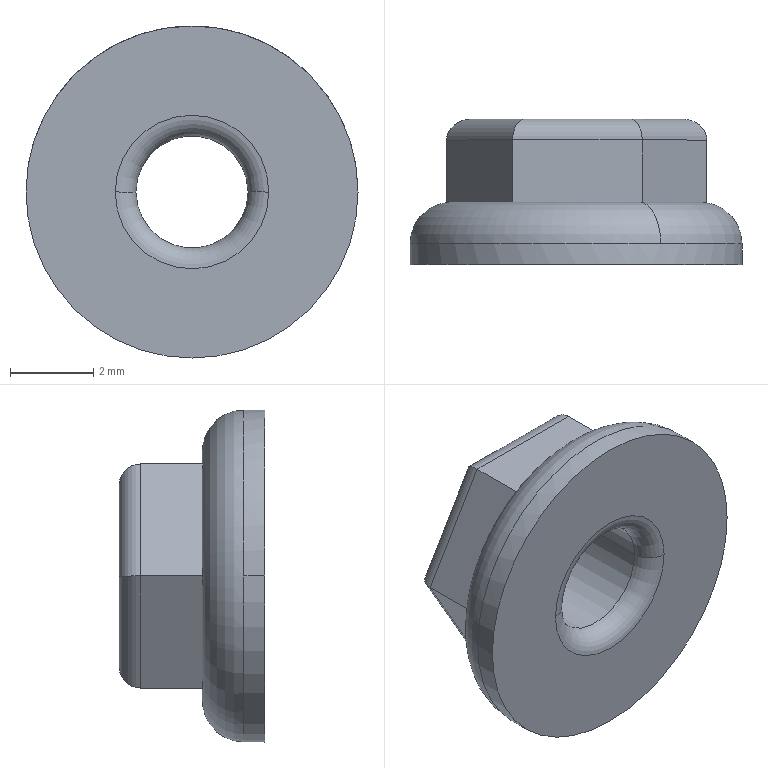Part | STEP file | FANGHUALUOMAO_3_1 | 1 solid | 30 faces | box 8 x 3.5 x 8 mm | volume 99.012 mm3 | plane 14 | cylinder 10 | torus 6 | commonest cylinder face diameters 1 x6 2.7 x2 8 x2
STEP:
#1=CARTESIAN_POINT('',(0.,0.,0.));
#2=DIRECTION('',(0.,0.,1.));
#3=DIRECTION('',(1.,0.,0.));
#4=AXIS2_PLACEMENT_3D('',#1,#2,#3);
#5=CARTESIAN_POINT('',(4.,0.,0.));
#6=VERTEX_POINT('',#5);
#7=CARTESIAN_POINT('',(-4.,0.,0.));
#8=VERTEX_POINT('',#7);
#9=CARTESIAN_POINT('',(0.,0.,0.));
#10=DIRECTION('',(0.,1.,0.));
#11=DIRECTION('',(1.,0.,0.));
#12=AXIS2_PLACEMENT_3D('',#9,#10,#11);
#13=CIRCLE('',#12,4.);
#14=EDGE_CURVE('',#6,#8,#13,.T.);
#15=ORIENTED_EDGE('',*,*,#14,.T.);
#16=CARTESIAN_POINT('',(0.,0.,0.));
#17=DIRECTION('',(0.,1.,0.));
#18=DIRECTION('',(-1.,0.,0.));
#19=AXIS2_PLACEMENT_3D('',#16,#17,#18);
#20=CIRCLE('',#19,4.);
#21=EDGE_CURVE('',#8,#6,#20,.T.);
#22=ORIENTED_EDGE('',*,*,#21,.T.);
#23=EDGE_LOOP('',(#15,#22));
#24=FACE_OUTER_BOUND('',#23,.F.);
#25=CARTESIAN_POINT('',(-1.85,0.,-0.02495));
#26=VERTEX_POINT('',#25);
#27=CARTESIAN_POINT('',(-1.85,0.,0.001234));
#28=VERTEX_POINT('',#27);
#29=CARTESIAN_POINT('',(0.,0.,0.));
#30=DIRECTION('',(0.,1.,0.));
#31=DIRECTION('',(-0.9999,0.,-0.01349));
#32=AXIS2_PLACEMENT_3D('',#29,#30,#31);
#33=CIRCLE('',#32,1.85);
#34=EDGE_CURVE('',#26,#28,#33,.T.);
#35=ORIENTED_EDGE('',*,*,#34,.F.);
#36=CARTESIAN_POINT('',(1.85,0.,-0.001234));
#37=VERTEX_POINT('',#36);
#38=CARTESIAN_POINT('',(0.,0.,0.));
#39=DIRECTION('',(0.,-1.,0.));
#40=DIRECTION('',(-0.9999,0.,-0.01349));
#41=AXIS2_PLACEMENT_3D('',#38,#39,#40);
#42=CIRCLE('',#41,1.85);
#43=EDGE_CURVE('',#26,#37,#42,.T.);
#44=ORIENTED_EDGE('',*,*,#43,.T.);
#45=CARTESIAN_POINT('',(1.85,0.,0.02495));
#46=VERTEX_POINT('',#45);
#47=CARTESIAN_POINT('',(0.,0.,0.));
#48=DIRECTION('',(0.,1.,0.));
#49=DIRECTION('',(0.9999,0.,0.01349));
#50=AXIS2_PLACEMENT_3D('',#47,#48,#49);
#51=CIRCLE('',#50,1.85);
#52=EDGE_CURVE('',#46,#37,#51,.T.);
#53=ORIENTED_EDGE('',*,*,#52,.F.);
#54=CARTESIAN_POINT('',(0.,0.,0.));
#55=DIRECTION('',(0.,-1.,0.));
#56=DIRECTION('',(0.9999,0.,0.01349));
#57=AXIS2_PLACEMENT_3D('',#54,#55,#56);
#58=CIRCLE('',#57,1.85);
#59=EDGE_CURVE('',#46,#28,#58,.T.);
#60=ORIENTED_EDGE('',*,*,#59,.T.);
#61=EDGE_LOOP('',(#35,#44,#53,#60));
#62=FACE_BOUND('',#61,.F.);
#63=CARTESIAN_POINT('',(0.,0.,0.));
#64=DIRECTION('',(0.,1.,0.));
#65=DIRECTION('',(1.,0.,0.));
#66=AXIS2_PLACEMENT_3D('',#63,#64,#65);
#67=PLANE('',#66);
#68=ADVANCED_FACE('',(#24,#62),#67,.F.);
#69=CARTESIAN_POINT('',(-4.,0.5,0.000001668));
#70=VERTEX_POINT('',#69);
#71=CARTESIAN_POINT('',(4.,0.5,0.));
#72=VERTEX_POINT('',#71);
#73=CARTESIAN_POINT('',(0.,0.5,0.));
#74=DIRECTION('',(0.,-1.,0.));
#75=DIRECTION('',(-1.,0.,0.000000417));
#76=AXIS2_PLACEMENT_3D('',#73,#74,#75);
#77=CIRCLE('',#76,4.);
#78=EDGE_CURVE('',#70,#72,#77,.T.);
#79=ORIENTED_EDGE('',*,*,#78,.F.);
#80=CARTESIAN_POINT('',(-4.,0.,0.000001112));
#81=DIRECTION('',(0.,1.,0.000001334));
#82=VECTOR('',#81,0.5);
#83=LINE('',#80,#82);
#84=EDGE_CURVE('',#8,#70,#83,.T.);
#85=ORIENTED_EDGE('',*,*,#84,.F.);
#86=ORIENTED_EDGE('',*,*,#14,.F.);
#87=CARTESIAN_POINT('',(4.,0.,0.));
#88=DIRECTION('',(0.,1.,0.00001117));
#89=VECTOR('',#88,0.5);
#90=LINE('',#87,#89);
#91=EDGE_CURVE('',#6,#72,#90,.T.);
#92=ORIENTED_EDGE('',*,*,#91,.T.);
#93=EDGE_LOOP('',(#79,#85,#86,#92));
#94=FACE_OUTER_BOUND('',#93,.F.);
#95=CARTESIAN_POINT('',(0.,0.,0.));
#96=DIRECTION('',(0.,1.,0.));
#97=DIRECTION('',(1.,0.,0.));
#98=AXIS2_PLACEMENT_3D('',#95,#96,#97);
#99=CYLINDRICAL_SURFACE('',#98,4.);
#100=ADVANCED_FACE('',(#94),#99,.T.);
#101=ORIENTED_EDGE('',*,*,#78,.T.);
#102=CARTESIAN_POINT('',(3.152,1.488,0.000008799));
#103=VERTEX_POINT('',#102);
#104=CARTESIAN_POINT('',(3.,0.5,0.000008374));
#105=DIRECTION('',(0.000002791,0.,-1.));
#106=DIRECTION('',(0.1523,0.9883,0.000000425));
#107=AXIS2_PLACEMENT_3D('',#104,#105,#106);
#108=CIRCLE('',#107,1.);
#109=EDGE_CURVE('',#103,#72,#108,.T.);
#110=ORIENTED_EDGE('',*,*,#109,.F.);
#111=CARTESIAN_POINT('',(2.987,1.5,-0.2804));
#112=VERTEX_POINT('',#111);
#113=CARTESIAN_POINT('',(3.005,1.5,-0.2493));
#114=CARTESIAN_POINT('',(3.042,1.499,-0.1872));
#115=CARTESIAN_POINT('',(3.097,1.496,-0.09395));
#116=CARTESIAN_POINT('',(3.134,1.491,-0.03136));
#117=CARTESIAN_POINT('',(3.152,1.488,0.000005525));
#118=B_SPLINE_CURVE_WITH_KNOTS('',3,(#111,#113,#114,#115,#116,#117),.UNSPECIFIED.,.F.,.F.,(4,1,1,4),(0.,0.3333,0.6667,1.),.UNSPECIFIED.);
#119=EDGE_CURVE('',#112,#103,#118,.T.);
#120=ORIENTED_EDGE('',*,*,#119,.F.);
#121=CARTESIAN_POINT('',(1.689,1.5,-2.479));
#122=VERTEX_POINT('',#121);
#123=CARTESIAN_POINT('',(0.,1.5,0.));
#124=DIRECTION('',(0.,-1.,0.));
#125=DIRECTION('',(0.563,0.,-0.8264));
#126=AXIS2_PLACEMENT_3D('',#123,#124,#125);
#127=CIRCLE('',#126,3.);
#128=EDGE_CURVE('',#122,#112,#127,.T.);
#129=ORIENTED_EDGE('',*,*,#128,.F.);
#130=CARTESIAN_POINT('',(1.559,1.493,-2.7));
#131=VERTEX_POINT('',#130);
#132=CARTESIAN_POINT('',(1.689,1.5,-2.479));
#133=CARTESIAN_POINT('',(1.674,1.5,-2.504));
#134=CARTESIAN_POINT('',(1.645,1.5,-2.554));
#135=CARTESIAN_POINT('',(1.602,1.497,-2.628));
#136=CARTESIAN_POINT('',(1.573,1.495,-2.676));
#137=B_SPLINE_CURVE_WITH_KNOTS('',3,(#132,#133,#134,#135,#136,#130),.UNSPECIFIED.,.F.,.F.,(4,1,1,4),(0.,0.3333,0.6667,1.),.UNSPECIFIED.);
#138=EDGE_CURVE('',#122,#131,#137,.T.);
#139=ORIENTED_EDGE('',*,*,#138,.T.);
#140=CARTESIAN_POINT('',(1.308,1.5,-2.7));
#141=VERTEX_POINT('',#140);
#142=CARTESIAN_POINT('',(1.335,1.5,-2.7));
#143=CARTESIAN_POINT('',(1.391,1.5,-2.7));
#144=CARTESIAN_POINT('',(1.475,1.497,-2.7));
#145=CARTESIAN_POINT('',(1.531,1.495,-2.7));
#146=CARTESIAN_POINT('',(1.559,1.493,-2.7));
#147=B_SPLINE_CURVE_WITH_KNOTS('',3,(#140,#142,#143,#144,#145,#146),.UNSPECIFIED.,.F.,.F.,(4,1,1,4),(0.,0.3333,0.6667,1.),.UNSPECIFIED.);
#148=EDGE_CURVE('',#141,#131,#147,.T.);
#149=ORIENTED_EDGE('',*,*,#148,.F.);
#150=CARTESIAN_POINT('',(-0.004458,1.5,-3.));
#151=VERTEX_POINT('',#150);
#152=CARTESIAN_POINT('',(0.,1.5,0.));
#153=DIRECTION('',(0.,-1.,0.));
#154=DIRECTION('',(-0.001486,0.,-1.));
#155=AXIS2_PLACEMENT_3D('',#152,#153,#154);
#156=CIRCLE('',#155,3.);
#157=EDGE_CURVE('',#151,#141,#156,.T.);
#158=ORIENTED_EDGE('',*,*,#157,.F.);
#159=CARTESIAN_POINT('',(-1.308,1.5,-2.7));
#160=VERTEX_POINT('',#159);
#161=CARTESIAN_POINT('',(0.,1.5,0.));
#162=DIRECTION('',(0.,-1.,0.));
#163=DIRECTION('',(-0.4359,0.,-0.9));
#164=AXIS2_PLACEMENT_3D('',#161,#162,#163);
#165=CIRCLE('',#164,3.);
#166=EDGE_CURVE('',#160,#151,#165,.T.);
#167=ORIENTED_EDGE('',*,*,#166,.F.);
#168=CARTESIAN_POINT('',(-1.559,1.493,-2.7));
#169=VERTEX_POINT('',#168);
#170=CARTESIAN_POINT('',(-1.531,1.495,-2.7));
#171=CARTESIAN_POINT('',(-1.475,1.497,-2.7));
#172=CARTESIAN_POINT('',(-1.391,1.5,-2.7));
#173=CARTESIAN_POINT('',(-1.335,1.5,-2.7));
#174=CARTESIAN_POINT('',(-1.308,1.5,-2.7));
#175=B_SPLINE_CURVE_WITH_KNOTS('',3,(#168,#170,#171,#172,#173,#174),.UNSPECIFIED.,.F.,.F.,(4,1,1,4),(0.,0.3333,0.6667,1.),.UNSPECIFIED.);
#176=EDGE_CURVE('',#169,#160,#175,.T.);
#177=ORIENTED_EDGE('',*,*,#176,.F.);
#178=CARTESIAN_POINT('',(-1.684,1.5,-2.482));
#179=VERTEX_POINT('',#178);
#180=CARTESIAN_POINT('',(-1.671,1.5,-2.507));
#181=CARTESIAN_POINT('',(-1.643,1.5,-2.555));
#182=CARTESIAN_POINT('',(-1.601,1.497,-2.627));
#183=CARTESIAN_POINT('',(-1.573,1.495,-2.676));
#184=CARTESIAN_POINT('',(-1.559,1.493,-2.7));
#185=B_SPLINE_CURVE_WITH_KNOTS('',3,(#178,#180,#181,#182,#183,#184),.UNSPECIFIED.,.F.,.F.,(4,1,1,4),(0.,0.3333,0.6667,1.),.UNSPECIFIED.);
#186=EDGE_CURVE('',#179,#169,#185,.T.);
#187=ORIENTED_EDGE('',*,*,#186,.F.);
#188=CARTESIAN_POINT('',(-2.992,1.5,-0.2175));
#189=VERTEX_POINT('',#188);
#190=CARTESIAN_POINT('',(0.,1.5,0.));
#191=DIRECTION('',(0.,-1.,0.));
#192=DIRECTION('',(-0.9974,0.,-0.07251));
#193=AXIS2_PLACEMENT_3D('',#190,#191,#192);
#194=CIRCLE('',#193,3.);
#195=EDGE_CURVE('',#189,#179,#194,.T.);
#196=ORIENTED_EDGE('',*,*,#195,.F.);
#197=CARTESIAN_POINT('',(-3.118,1.493,0.0002294));
#198=VERTEX_POINT('',#197);
#199=CARTESIAN_POINT('',(-3.104,1.495,-0.0243));
#200=CARTESIAN_POINT('',(-3.075,1.497,-0.07314));
#201=CARTESIAN_POINT('',(-3.034,1.5,-0.1456));
#202=CARTESIAN_POINT('',(-3.006,1.5,-0.1936));
#203=CARTESIAN_POINT('',(-2.992,1.5,-0.2175));
#204=B_SPLINE_CURVE_WITH_KNOTS('',3,(#197,#199,#200,#201,#202,#203),.UNSPECIFIED.,.F.,.F.,(4,1,1,4),(0.,0.3333,0.6667,1.),.UNSPECIFIED.);
#205=EDGE_CURVE('',#198,#189,#204,.T.);
#206=ORIENTED_EDGE('',*,*,#205,.F.);
#207=CARTESIAN_POINT('',(-2.992,1.5,0.2127));
#208=VERTEX_POINT('',#207);
#209=CARTESIAN_POINT('',(-3.006,1.5,0.1891));
#210=CARTESIAN_POINT('',(-3.034,1.5,0.1418));
#211=CARTESIAN_POINT('',(-3.076,1.497,0.07108));
#212=CARTESIAN_POINT('',(-3.104,1.495,0.02384));
#213=CARTESIAN_POINT('',(-3.118,1.493,0.0002294));
#214=B_SPLINE_CURVE_WITH_KNOTS('',3,(#207,#209,#210,#211,#212,#213),.UNSPECIFIED.,.F.,.F.,(4,1,1,4),(0.,0.3333,0.6667,1.),.UNSPECIFIED.);
#215=EDGE_CURVE('',#208,#198,#214,.T.);
#216=ORIENTED_EDGE('',*,*,#215,.F.);
#217=CARTESIAN_POINT('',(-1.633,1.5,2.517));
#218=VERTEX_POINT('',#217);
#219=CARTESIAN_POINT('',(0.,1.5,0.));
#220=DIRECTION('',(0.,-1.,0.));
#221=DIRECTION('',(-0.5442,0.,0.839));
#222=AXIS2_PLACEMENT_3D('',#219,#220,#221);
#223=CIRCLE('',#222,3.);
#224=EDGE_CURVE('',#218,#208,#223,.T.);
#225=ORIENTED_EDGE('',*,*,#224,.F.);
#226=CARTESIAN_POINT('',(-1.524,1.495,2.7));
#227=VERTEX_POINT('',#226);
#228=CARTESIAN_POINT('',(-1.537,1.496,2.679));
#229=CARTESIAN_POINT('',(-1.561,1.498,2.638));
#230=CARTESIAN_POINT('',(-1.597,1.5,2.577));
#231=CARTESIAN_POINT('',(-1.621,1.5,2.537));
#232=CARTESIAN_POINT('',(-1.633,1.5,2.517));
#233=B_SPLINE_CURVE_WITH_KNOTS('',3,(#226,#228,#229,#230,#231,#232),.UNSPECIFIED.,.F.,.F.,(4,1,1,4),(0.,0.3333,0.6667,1.),.UNSPECIFIED.);
#234=EDGE_CURVE('',#227,#218,#233,.T.);
#235=ORIENTED_EDGE('',*,*,#234,.F.);
#236=CARTESIAN_POINT('',(-1.308,1.5,2.7));
#237=VERTEX_POINT('',#236);
#238=CARTESIAN_POINT('',(-1.524,1.495,2.7));
#239=CARTESIAN_POINT('',(-1.501,1.496,2.7));
#240=CARTESIAN_POINT('',(-1.453,1.498,2.7));
#241=CARTESIAN_POINT('',(-1.381,1.5,2.7));
#242=CARTESIAN_POINT('',(-1.332,1.5,2.7));
#243=B_SPLINE_CURVE_WITH_KNOTS('',3,(#238,#239,#240,#241,#242,#236),.UNSPECIFIED.,.F.,.F.,(4,1,1,4),(0.,0.3333,0.6667,1.),.UNSPECIFIED.);
#244=EDGE_CURVE('',#227,#237,#243,.T.);
#245=ORIENTED_EDGE('',*,*,#244,.T.);
#246=CARTESIAN_POINT('',(0.004458,1.5,3.));
#247=VERTEX_POINT('',#246);
#248=CARTESIAN_POINT('',(0.,1.5,0.));
#249=DIRECTION('',(0.,-1.,0.));
#250=DIRECTION('',(0.001486,0.,1.));
#251=AXIS2_PLACEMENT_3D('',#248,#249,#250);
#252=CIRCLE('',#251,3.);
#253=EDGE_CURVE('',#247,#237,#252,.T.);
#254=ORIENTED_EDGE('',*,*,#253,.F.);
#255=CARTESIAN_POINT('',(1.308,1.5,2.7));
#256=VERTEX_POINT('',#255);
#257=CARTESIAN_POINT('',(0.,1.5,0.));
#258=DIRECTION('',(0.,-1.,0.));
#259=DIRECTION('',(0.4359,0.,0.9));
#260=AXIS2_PLACEMENT_3D('',#257,#258,#259);
#261=CIRCLE('',#260,3.);
#262=EDGE_CURVE('',#256,#247,#261,.T.);
#263=ORIENTED_EDGE('',*,*,#262,.F.);
#264=CARTESIAN_POINT('',(1.593,1.491,2.7));
#265=VERTEX_POINT('',#264);
#266=CARTESIAN_POINT('',(1.561,1.493,2.7));
#267=CARTESIAN_POINT('',(1.498,1.497,2.7));
#268=CARTESIAN_POINT('',(1.402,1.499,2.7));
#269=CARTESIAN_POINT('',(1.339,1.5,2.7));
#270=CARTESIAN_POINT('',(1.308,1.5,2.7));
#271=B_SPLINE_CURVE_WITH_KNOTS('',3,(#264,#266,#267,#268,#269,#270),.UNSPECIFIED.,.F.,.F.,(4,1,1,4),(0.,0.3333,0.6667,1.),.UNSPECIFIED.);
#272=EDGE_CURVE('',#265,#256,#271,.T.);
#273=ORIENTED_EDGE('',*,*,#272,.F.);
#274=CARTESIAN_POINT('',(1.597,1.491,2.693));
#275=VERTEX_POINT('',#274);
#276=CARTESIAN_POINT('',(1.597,1.491,2.694));
#277=CARTESIAN_POINT('',(1.596,1.491,2.695));
#278=CARTESIAN_POINT('',(1.595,1.491,2.698));
#279=CARTESIAN_POINT('',(1.594,1.491,2.699));
#280=CARTESIAN_POINT('',(1.593,1.491,2.7));
#281=B_SPLINE_CURVE_WITH_KNOTS('',3,(#274,#276,#277,#278,#279,#280),.UNSPECIFIED.,.F.,.F.,(4,1,1,4),(0.,0.3333,0.6667,1.),.UNSPECIFIED.);
#282=EDGE_CURVE('',#275,#265,#281,.T.);
#283=ORIENTED_EDGE('',*,*,#282,.F.);
#284=CARTESIAN_POINT('',(2.041,0.5,3.44));
#285=VERTEX_POINT('',#284);
#286=CARTESIAN_POINT('',(1.53,0.5,2.58));
#287=DIRECTION('',(0.8601,0.,-0.5101));
#288=DIRECTION('',(0.06699,0.9913,0.1129));
#289=AXIS2_PLACEMENT_3D('',#286,#287,#288);
#290=CIRCLE('',#289,1.);
#291=EDGE_CURVE('',#275,#285,#290,.T.);
#292=ORIENTED_EDGE('',*,*,#291,.T.);
#293=CARTESIAN_POINT('',(0.,0.5,0.));
#294=DIRECTION('',(0.,-1.,0.));
#295=DIRECTION('',(0.5101,0.,0.8601));
#296=AXIS2_PLACEMENT_3D('',#293,#294,#295);
#297=CIRCLE('',#296,4.);
#298=EDGE_CURVE('',#285,#70,#297,.T.);
#299=ORIENTED_EDGE('',*,*,#298,.T.);
#300=EDGE_LOOP('',(#101,#110,#120,#129,#139,#149,#158,#167,#177,#187,#196,#206,#216,#225,#235,#245,#254,#263,#273,#283,#292,#299));
#301=FACE_OUTER_BOUND('',#300,.F.);
#302=CARTESIAN_POINT('',(0.,0.5,0.));
#303=DIRECTION('',(0.,1.,0.));
#304=DIRECTION('',(-0.001486,0.,-1.));
#305=AXIS2_PLACEMENT_3D('',#302,#303,#304);
#306=TOROIDAL_SURFACE('',#305,3.,1.);
#307=ADVANCED_FACE('',(#301),#306,.T.);
#308=CARTESIAN_POINT('',(0.,0.5,0.));
#309=DIRECTION('',(0.,-1.,0.));
#310=DIRECTION('',(1.,0.,0.));
#311=AXIS2_PLACEMENT_3D('',#308,#309,#310);
#312=CIRCLE('',#311,4.);
#313=EDGE_CURVE('',#72,#285,#312,.T.);
#314=ORIENTED_EDGE('',*,*,#313,.T.);
#315=ORIENTED_EDGE('',*,*,#291,.F.);
#316=CARTESIAN_POINT('',(1.742,1.5,2.442));
#317=VERTEX_POINT('',#316);
#318=CARTESIAN_POINT('',(1.726,1.5,2.47));
#319=CARTESIAN_POINT('',(1.694,1.499,2.526));
#320=CARTESIAN_POINT('',(1.646,1.497,2.609));
#321=CARTESIAN_POINT('',(1.614,1.493,2.665));
#322=CARTESIAN_POINT('',(1.597,1.491,2.693));
#323=B_SPLINE_CURVE_WITH_KNOTS('',3,(#316,#318,#319,#320,#321,#322),.UNSPECIFIED.,.F.,.F.,(4,1,1,4),(0.,0.3333,0.6667,1.),.UNSPECIFIED.);
#324=EDGE_CURVE('',#317,#275,#323,.T.);
#325=ORIENTED_EDGE('',*,*,#324,.F.);
#326=CARTESIAN_POINT('',(2.986,1.5,0.2878));
#327=VERTEX_POINT('',#326);
#328=CARTESIAN_POINT('',(0.,1.5,0.));
#329=DIRECTION('',(0.,-1.,0.));
#330=DIRECTION('',(0.9954,0.,0.09594));
#331=AXIS2_PLACEMENT_3D('',#328,#329,#330);
#332=CIRCLE('',#331,3.);
#333=EDGE_CURVE('',#327,#317,#332,.T.);
#334=ORIENTED_EDGE('',*,*,#333,.F.);
#335=CARTESIAN_POINT('',(3.152,1.488,0.000005525));
#336=CARTESIAN_POINT('',(3.134,1.491,0.03193));
#337=CARTESIAN_POINT('',(3.097,1.496,0.09583));
#338=CARTESIAN_POINT('',(3.042,1.499,0.1917));
#339=CARTESIAN_POINT('',(3.005,1.5,0.2558));
#340=CARTESIAN_POINT('',(2.986,1.5,0.2878));
#341=B_SPLINE_CURVE_WITH_KNOTS('',3,(#335,#336,#337,#338,#339,#340),.UNSPECIFIED.,.F.,.F.,(4,1,1,4),(0.,0.3333,0.6667,1.),.UNSPECIFIED.);
#342=EDGE_CURVE('',#103,#327,#341,.T.);
#343=ORIENTED_EDGE('',*,*,#342,.F.);
#344=ORIENTED_EDGE('',*,*,#109,.T.);
#345=EDGE_LOOP('',(#314,#315,#325,#334,#343,#344));
#346=FACE_OUTER_BOUND('',#345,.F.);
#347=CARTESIAN_POINT('',(0.,0.5,0.));
#348=DIRECTION('',(0.,1.,0.));
#349=DIRECTION('',(-0.001486,0.,-1.));
#350=AXIS2_PLACEMENT_3D('',#347,#348,#349);
#351=TOROIDAL_SURFACE('',#350,3.,1.);
#352=ADVANCED_FACE('',(#346),#351,.T.);
#353=ORIENTED_EDGE('',*,*,#313,.F.);
#354=ORIENTED_EDGE('',*,*,#91,.F.);
#355=ORIENTED_EDGE('',*,*,#21,.F.);
#356=ORIENTED_EDGE('',*,*,#84,.T.);
#357=ORIENTED_EDGE('',*,*,#298,.F.);
#358=EDGE_LOOP('',(#353,#354,#355,#356,#357));
#359=FACE_OUTER_BOUND('',#358,.F.);
#360=CARTESIAN_POINT('',(0.,0.,0.));
#361=DIRECTION('',(0.,1.,0.));
#362=DIRECTION('',(1.,0.,0.));
#363=AXIS2_PLACEMENT_3D('',#360,#361,#362);
#364=CYLINDRICAL_SURFACE('',#363,4.);
#365=ADVANCED_FACE('',(#359),#364,.T.);
#366=CARTESIAN_POINT('',(3.152,3.,0.000001431));
#367=VERTEX_POINT('',#366);
#368=CARTESIAN_POINT('',(3.152,1.488,0.000005525));
#369=DIRECTION('',(0.000000206,1.,-0.000002708));
#370=VECTOR('',#369,1.512);
#371=LINE('',#368,#370);
#372=EDGE_CURVE('',#103,#367,#371,.T.);
#373=ORIENTED_EDGE('',*,*,#372,.F.);
#374=ORIENTED_EDGE('',*,*,#342,.T.);
#375=CARTESIAN_POINT('',(1.742,1.5,2.442));
#376=DIRECTION('',(0.5,0.,-0.866));
#377=VECTOR('',#376,2.488);
#378=LINE('',#375,#377);
#379=EDGE_CURVE('',#317,#327,#378,.T.);
#380=ORIENTED_EDGE('',*,*,#379,.F.);
#381=ORIENTED_EDGE('',*,*,#324,.T.);
#382=ORIENTED_EDGE('',*,*,#282,.T.);
#383=CARTESIAN_POINT('',(1.593,3.,2.7));
#384=VERTEX_POINT('',#383);
#385=CARTESIAN_POINT('',(1.593,1.491,2.7));
#386=DIRECTION('',(0.000001295,1.,0.000002194));
#387=VECTOR('',#386,1.509);
#388=LINE('',#385,#387);
#389=EDGE_CURVE('',#265,#384,#388,.T.);
#390=ORIENTED_EDGE('',*,*,#389,.T.);
#391=CARTESIAN_POINT('',(3.152,3.,0.000001431));
#392=DIRECTION('',(-0.5,0.,0.866));
#393=VECTOR('',#392,3.118);
#394=LINE('',#391,#393);
#395=EDGE_CURVE('',#367,#384,#394,.T.);
#396=ORIENTED_EDGE('',*,*,#395,.F.);
#397=EDGE_LOOP('',(#373,#374,#380,#381,#382,#390,#396));
#398=FACE_OUTER_BOUND('',#397,.F.);
#399=CARTESIAN_POINT('',(1.593,1.5,2.7));
#400=DIRECTION('',(0.866,0.,0.5));
#401=DIRECTION('',(0.5,0.,-0.866));
#402=AXIS2_PLACEMENT_3D('',#399,#400,#401);
#403=PLANE('',#402);
#404=ADVANCED_FACE('',(#398),#403,.T.);
#405=CARTESIAN_POINT('',(1.559,3.,-2.7));
#406=VERTEX_POINT('',#405);
#407=CARTESIAN_POINT('',(1.559,1.493,-2.7));
#408=DIRECTION('',(0.,1.,0.));
#409=VECTOR('',#408,1.507);
#410=LINE('',#407,#409);
#411=EDGE_CURVE('',#131,#406,#410,.T.);
#412=ORIENTED_EDGE('',*,*,#411,.F.);
#413=ORIENTED_EDGE('',*,*,#138,.F.);
#414=CARTESIAN_POINT('',(2.987,1.5,-0.2804));
#415=DIRECTION('',(-0.5083,0.,-0.8612));
#416=VECTOR('',#415,2.553);
#417=LINE('',#414,#416);
#418=EDGE_CURVE('',#112,#122,#417,.T.);
#419=ORIENTED_EDGE('',*,*,#418,.F.);
#420=ORIENTED_EDGE('',*,*,#119,.T.);
#421=ORIENTED_EDGE('',*,*,#372,.T.);
#422=CARTESIAN_POINT('',(1.559,3.,-2.7));
#423=DIRECTION('',(0.5083,0.,0.8612));
#424=VECTOR('',#423,3.135);
#425=LINE('',#422,#424);
#426=EDGE_CURVE('',#406,#367,#425,.T.);
#427=ORIENTED_EDGE('',*,*,#426,.F.);
#428=EDGE_LOOP('',(#412,#413,#419,#420,#421,#427));
#429=FACE_OUTER_BOUND('',#428,.F.);
#430=CARTESIAN_POINT('',(3.152,1.5,0.));
#431=DIRECTION('',(0.8612,0.,-0.5083));
#432=DIRECTION('',(-0.5083,0.,-0.8612));
#433=AXIS2_PLACEMENT_3D('',#430,#431,#432);
#434=PLANE('',#433);
#435=ADVANCED_FACE('',(#429),#434,.T.);
#436=CARTESIAN_POINT('',(-1.559,3.,-2.7));
#437=VERTEX_POINT('',#436);
#438=CARTESIAN_POINT('',(-1.559,1.493,-2.7));
#439=DIRECTION('',(-0.000000306,1.,0.000000029));
#440=VECTOR('',#439,1.507);
#441=LINE('',#438,#440);
#442=EDGE_CURVE('',#169,#437,#441,.T.);
#443=ORIENTED_EDGE('',*,*,#442,.F.);
#444=ORIENTED_EDGE('',*,*,#176,.T.);
#445=CARTESIAN_POINT('',(1.308,1.5,-2.7));
#446=DIRECTION('',(-1.,0.,0.000000015));
#447=VECTOR('',#446,2.615);
#448=LINE('',#445,#447);
#449=EDGE_CURVE('',#141,#160,#448,.T.);
#450=ORIENTED_EDGE('',*,*,#449,.F.);
#451=ORIENTED_EDGE('',*,*,#148,.T.);
#452=ORIENTED_EDGE('',*,*,#411,.T.);
#453=CARTESIAN_POINT('',(-1.559,3.,-2.7));
#454=DIRECTION('',(1.,0.,0.00000007));
#455=VECTOR('',#454,3.118);
#456=LINE('',#453,#455);
#457=EDGE_CURVE('',#437,#406,#456,.T.);
#458=ORIENTED_EDGE('',*,*,#457,.F.);
#459=EDGE_LOOP('',(#443,#444,#450,#451,#452,#458));
#460=FACE_OUTER_BOUND('',#459,.F.);
#461=CARTESIAN_POINT('',(1.559,1.5,-2.7));
#462=DIRECTION('',(0.,0.,-1.));
#463=DIRECTION('',(-1.,0.,0.));
#464=AXIS2_PLACEMENT_3D('',#461,#462,#463);
#465=PLANE('',#464);
#466=ADVANCED_FACE('',(#460),#465,.T.);
#467=CARTESIAN_POINT('',(-3.118,3.,0.0002368));
#468=VERTEX_POINT('',#467);
#469=CARTESIAN_POINT('',(-3.118,3.,0.0002368));
#470=DIRECTION('',(0.000002242,-1.,-0.000004906));
#471=VECTOR('',#470,1.507);
#472=LINE('',#469,#471);
#473=EDGE_CURVE('',#468,#198,#472,.T.);
#474=ORIENTED_EDGE('',*,*,#473,.T.);
#475=ORIENTED_EDGE('',*,*,#205,.T.);
#476=CARTESIAN_POINT('',(-1.684,1.5,-2.482));
#477=DIRECTION('',(-0.5,0.,0.866));
#478=VECTOR('',#477,2.615);
#479=LINE('',#476,#478);
#480=EDGE_CURVE('',#179,#189,#479,.T.);
#481=ORIENTED_EDGE('',*,*,#480,.F.);
#482=ORIENTED_EDGE('',*,*,#186,.T.);
#483=ORIENTED_EDGE('',*,*,#442,.T.);
#484=CARTESIAN_POINT('',(-3.118,3.,0.0002368));
#485=DIRECTION('',(0.5,0.,-0.866));
#486=VECTOR('',#485,3.118);
#487=LINE('',#484,#486);
#488=EDGE_CURVE('',#468,#437,#487,.T.);
#489=ORIENTED_EDGE('',*,*,#488,.F.);
#490=EDGE_LOOP('',(#474,#475,#481,#482,#483,#489));
#491=FACE_OUTER_BOUND('',#490,.F.);
#492=CARTESIAN_POINT('',(-1.559,1.5,-2.7));
#493=DIRECTION('',(-0.866,0.,-0.5));
#494=DIRECTION('',(-0.5,0.,0.866));
#495=AXIS2_PLACEMENT_3D('',#492,#493,#494);
#496=PLANE('',#495);
#497=ADVANCED_FACE('',(#491),#496,.T.);
#498=CARTESIAN_POINT('',(-2.992,1.5,0.2127));
#499=DIRECTION('',(0.5083,0.,0.8612));
#500=VECTOR('',#499,2.676);
#501=LINE('',#498,#500);
#502=EDGE_CURVE('',#208,#218,#501,.T.);
#503=ORIENTED_EDGE('',*,*,#502,.F.);
#504=ORIENTED_EDGE('',*,*,#215,.T.);
#505=ORIENTED_EDGE('',*,*,#473,.F.);
#506=CARTESIAN_POINT('',(-1.524,3.,2.7));
#507=VERTEX_POINT('',#506);
#508=CARTESIAN_POINT('',(-1.524,3.,2.7));
#509=DIRECTION('',(-0.5083,0.,-0.8612));
#510=VECTOR('',#509,3.135);
#511=LINE('',#508,#510);
#512=EDGE_CURVE('',#507,#468,#511,.T.);
#513=ORIENTED_EDGE('',*,*,#512,.F.);
#514=CARTESIAN_POINT('',(-1.524,1.495,2.7));
#515=DIRECTION('',(0.,1.,0.));
#516=VECTOR('',#515,1.505);
#517=LINE('',#514,#516);
#518=EDGE_CURVE('',#227,#507,#517,.T.);
#519=ORIENTED_EDGE('',*,*,#518,.F.);
#520=ORIENTED_EDGE('',*,*,#234,.T.);
#521=EDGE_LOOP('',(#503,#504,#505,#513,#519,#520));
#522=FACE_OUTER_BOUND('',#521,.F.);
#523=CARTESIAN_POINT('',(-3.118,1.5,0.0002459));
#524=DIRECTION('',(-0.8612,0.,0.5083));
#525=DIRECTION('',(0.5083,0.,0.8612));
#526=AXIS2_PLACEMENT_3D('',#523,#524,#525);
#527=PLANE('',#526);
#528=ADVANCED_FACE('',(#522),#527,.T.);
#529=ORIENTED_EDGE('',*,*,#224,.T.);
#530=ORIENTED_EDGE('',*,*,#502,.T.);
#531=EDGE_LOOP('',(#529,#530));
#532=FACE_OUTER_BOUND('',#531,.F.);
#533=CARTESIAN_POINT('',(0.,1.5,0.));
#534=DIRECTION('',(0.,1.,0.));
#535=DIRECTION('',(1.,0.,0.));
#536=AXIS2_PLACEMENT_3D('',#533,#534,#535);
#537=PLANE('',#536);
#538=ADVANCED_FACE('',(#532),#537,.T.);
#539=ORIENTED_EDGE('',*,*,#512,.T.);
#540=CARTESIAN_POINT('',(-2.539,3.5,-0.002524));
#541=VERTEX_POINT('',#540);
#542=CARTESIAN_POINT('',(-3.118,3.,0.0002368));
#543=CARTESIAN_POINT('',(-3.118,3.03,0.0002368));
#544=CARTESIAN_POINT('',(-3.112,3.092,0.0002153));
#545=CARTESIAN_POINT('',(-3.079,3.189,0.00007731));
#546=CARTESIAN_POINT('',(-3.026,3.276,-0.0002292));
#547=CARTESIAN_POINT('',(-2.962,3.346,-0.000467));
#548=CARTESIAN_POINT('',(-2.863,3.418,-0.0009873));
#549=CARTESIAN_POINT('',(-2.772,3.46,-0.001404));
#550=CARTESIAN_POINT('',(-2.665,3.492,-0.001922));
#551=CARTESIAN_POINT('',(-2.583,3.5,-0.002315));
#552=B_SPLINE_CURVE_WITH_KNOTS('',3,(#542,#543,#544,#545,#546,#547,#548,#549,#550,#551,#540),.UNSPECIFIED.,.F.,.F.,(4,1,1,1,1,1,1,1,4),(0.,0.125,0.25,0.375,0.5,0.625,0.75,0.875,1.),.UNSPECIFIED.);
#553=EDGE_CURVE('',#468,#541,#552,.T.);
#554=ORIENTED_EDGE('',*,*,#553,.T.);
#555=CARTESIAN_POINT('',(-1.239,3.5,2.2));
#556=VERTEX_POINT('',#555);
#557=CARTESIAN_POINT('',(-1.239,3.5,2.2));
#558=DIRECTION('',(-0.5083,0.,-0.8612));
#559=VECTOR('',#558,2.558);
#560=LINE('',#557,#559);
#561=EDGE_CURVE('',#556,#541,#560,.T.);
#562=ORIENTED_EDGE('',*,*,#561,.F.);
#563=CARTESIAN_POINT('',(-1.524,3.,2.7));
#564=CARTESIAN_POINT('',(-1.524,3.03,2.7));
#565=CARTESIAN_POINT('',(-1.521,3.092,2.695));
#566=CARTESIAN_POINT('',(-1.505,3.189,2.667));
#567=CARTESIAN_POINT('',(-1.479,3.276,2.62));
#568=CARTESIAN_POINT('',(-1.447,3.347,2.565));
#569=CARTESIAN_POINT('',(-1.399,3.418,2.48));
#570=CARTESIAN_POINT('',(-1.354,3.461,2.401));
#571=CARTESIAN_POINT('',(-1.301,3.492,2.309));
#572=CARTESIAN_POINT('',(-1.26,3.5,2.237));
#573=CARTESIAN_POINT('',(-1.239,3.5,2.2));
#574=B_SPLINE_CURVE_WITH_KNOTS('',3,(#563,#564,#565,#566,#567,#568,#569,#570,#571,#572,#573),.UNSPECIFIED.,.F.,.F.,(4,1,1,1,1,1,1,1,4),(0.,0.125,0.25,0.375,0.5,0.625,0.75,0.875,1.),.UNSPECIFIED.);
#575=EDGE_CURVE('',#507,#556,#574,.T.);
#576=ORIENTED_EDGE('',*,*,#575,.F.);
#577=EDGE_LOOP('',(#539,#554,#562,#576));
#578=FACE_OUTER_BOUND('',#577,.F.);
#579=CARTESIAN_POINT('',(-11.053,3.,-14.429));
#580=DIRECTION('',(0.5083,0.,0.8612));
#581=DIRECTION('',(0.,1.,0.));
#582=AXIS2_PLACEMENT_3D('',#579,#580,#581);
#583=CYLINDRICAL_SURFACE('',#582,0.5);
#584=ADVANCED_FACE('',(#578),#583,.T.);
#585=ORIENTED_EDGE('',*,*,#488,.T.);
#586=CARTESIAN_POINT('',(-1.27,3.5,-2.2));
#587=VERTEX_POINT('',#586);
#588=CARTESIAN_POINT('',(-1.559,3.,-2.7));
#589=CARTESIAN_POINT('',(-1.559,3.03,-2.7));
#590=CARTESIAN_POINT('',(-1.556,3.092,-2.695));
#591=CARTESIAN_POINT('',(-1.54,3.189,-2.667));
#592=CARTESIAN_POINT('',(-1.513,3.276,-2.62));
#593=CARTESIAN_POINT('',(-1.481,3.347,-2.565));
#594=CARTESIAN_POINT('',(-1.432,3.418,-2.48));
#595=CARTESIAN_POINT('',(-1.386,3.461,-2.401));
#596=CARTESIAN_POINT('',(-1.333,3.492,-2.309));
#597=CARTESIAN_POINT('',(-1.292,3.5,-2.238));
#598=B_SPLINE_CURVE_WITH_KNOTS('',3,(#588,#589,#590,#591,#592,#593,#594,#595,#596,#597,#586),.UNSPECIFIED.,.F.,.F.,(4,1,1,1,1,1,1,1,4),(0.,0.125,0.25,0.375,0.5,0.625,0.75,0.875,1.),.UNSPECIFIED.);
#599=EDGE_CURVE('',#437,#587,#598,.T.);
#600=ORIENTED_EDGE('',*,*,#599,.T.);
#601=CARTESIAN_POINT('',(-2.539,3.5,-0.002524));
#602=DIRECTION('',(0.5,0.,-0.866));
#603=VECTOR('',#602,2.537);
#604=LINE('',#601,#603);
#605=EDGE_CURVE('',#541,#587,#604,.T.);
#606=ORIENTED_EDGE('',*,*,#605,.F.);
#607=ORIENTED_EDGE('',*,*,#553,.F.);
#608=EDGE_LOOP('',(#585,#600,#606,#607));
#609=FACE_OUTER_BOUND('',#608,.F.);
#610=CARTESIAN_POINT('',(5.79,3.,-14.429));
#611=DIRECTION('',(-0.5,0.,0.866));
#612=DIRECTION('',(0.,1.,0.));
#613=AXIS2_PLACEMENT_3D('',#610,#611,#612);
#614=CYLINDRICAL_SURFACE('',#613,0.5);
#615=ADVANCED_FACE('',(#609),#614,.T.);
#616=CARTESIAN_POINT('',(1.273,3.5,-2.2));
#617=VERTEX_POINT('',#616);
#618=CARTESIAN_POINT('',(1.273,3.5,-2.2));
#619=DIRECTION('',(-1.,0.,0.));
#620=VECTOR('',#619,2.544);
#621=LINE('',#618,#620);
#622=EDGE_CURVE('',#617,#587,#621,.T.);
#623=ORIENTED_EDGE('',*,*,#622,.T.);
#624=ORIENTED_EDGE('',*,*,#599,.F.);
#625=ORIENTED_EDGE('',*,*,#457,.T.);
#626=CARTESIAN_POINT('',(1.559,3.,-2.7));
#627=CARTESIAN_POINT('',(1.559,3.03,-2.7));
#628=CARTESIAN_POINT('',(1.556,3.092,-2.695));
#629=CARTESIAN_POINT('',(1.54,3.189,-2.667));
#630=CARTESIAN_POINT('',(1.513,3.276,-2.62));
#631=CARTESIAN_POINT('',(1.482,3.347,-2.565));
#632=CARTESIAN_POINT('',(1.433,3.418,-2.48));
#633=CARTESIAN_POINT('',(1.388,3.461,-2.401));
#634=CARTESIAN_POINT('',(1.336,3.492,-2.309));
#635=CARTESIAN_POINT('',(1.295,3.5,-2.237));
#636=CARTESIAN_POINT('',(1.273,3.5,-2.2));
#637=B_SPLINE_CURVE_WITH_KNOTS('',3,(#626,#627,#628,#629,#630,#631,#632,#633,#634,#635,#636),.UNSPECIFIED.,.F.,.F.,(4,1,1,1,1,1,1,1,4),(0.,0.125,0.25,0.375,0.5,0.625,0.75,0.875,1.),.UNSPECIFIED.);
#638=EDGE_CURVE('',#406,#617,#637,.T.);
#639=ORIENTED_EDGE('',*,*,#638,.T.);
#640=EDGE_LOOP('',(#623,#624,#625,#639));
#641=FACE_OUTER_BOUND('',#640,.F.);
#642=CARTESIAN_POINT('',(14.429,3.,-2.2));
#643=DIRECTION('',(-1.,0.,0.));
#644=DIRECTION('',(0.,1.,0.));
#645=AXIS2_PLACEMENT_3D('',#642,#643,#644);
#646=CYLINDRICAL_SURFACE('',#645,0.5);
#647=ADVANCED_FACE('',(#641),#646,.T.);
#648=CARTESIAN_POINT('',(2.573,3.5,0.00277));
#649=VERTEX_POINT('',#648);
#650=CARTESIAN_POINT('',(1.305,3.5,2.2));
#651=VERTEX_POINT('',#650);
#652=CARTESIAN_POINT('',(2.573,3.5,0.00277));
#653=DIRECTION('',(-0.5,0.,0.866));
#654=VECTOR('',#653,2.537);
#655=LINE('',#652,#654);
#656=EDGE_CURVE('',#649,#651,#655,.T.);
#657=ORIENTED_EDGE('',*,*,#656,.T.);
#658=CARTESIAN_POINT('',(-1.239,3.5,2.2));
#659=DIRECTION('',(1.,0.,0.));
#660=VECTOR('',#659,2.544);
#661=LINE('',#658,#660);
#662=EDGE_CURVE('',#556,#651,#661,.T.);
#663=ORIENTED_EDGE('',*,*,#662,.F.);
#664=ORIENTED_EDGE('',*,*,#561,.T.);
#665=ORIENTED_EDGE('',*,*,#605,.T.);
#666=ORIENTED_EDGE('',*,*,#622,.F.);
#667=CARTESIAN_POINT('',(1.273,3.5,-2.2));
#668=DIRECTION('',(0.5083,0.,0.8612));
#669=VECTOR('',#668,2.558);
#670=LINE('',#667,#669);
#671=EDGE_CURVE('',#617,#649,#670,.T.);
#672=ORIENTED_EDGE('',*,*,#671,.T.);
#673=EDGE_LOOP('',(#657,#663,#664,#665,#666,#672));
#674=FACE_OUTER_BOUND('',#673,.F.);
#675=CARTESIAN_POINT('',(1.85,3.5,-0.03545));
#676=VERTEX_POINT('',#675);
#677=CARTESIAN_POINT('',(1.85,3.5,0.));
#678=VERTEX_POINT('',#677);
#679=CARTESIAN_POINT('',(0.,3.5,0.));
#680=DIRECTION('',(0.,-1.,0.));
#681=DIRECTION('',(0.9998,0.,-0.01916));
#682=AXIS2_PLACEMENT_3D('',#679,#680,#681);
#683=CIRCLE('',#682,1.85);
#684=EDGE_CURVE('',#676,#678,#683,.T.);
#685=ORIENTED_EDGE('',*,*,#684,.F.);
#686=CARTESIAN_POINT('',(-1.85,3.5,0.));
#687=VERTEX_POINT('',#686);
#688=CARTESIAN_POINT('',(0.,3.5,0.));
#689=DIRECTION('',(0.,1.,0.));
#690=DIRECTION('',(0.9998,0.,-0.01916));
#691=AXIS2_PLACEMENT_3D('',#688,#689,#690);
#692=CIRCLE('',#691,1.85);
#693=EDGE_CURVE('',#676,#687,#692,.T.);
#694=ORIENTED_EDGE('',*,*,#693,.T.);
#695=CARTESIAN_POINT('',(-1.85,3.5,0.03545));
#696=VERTEX_POINT('',#695);
#697=CARTESIAN_POINT('',(0.,3.5,0.));
#698=DIRECTION('',(0.,-1.,0.));
#699=DIRECTION('',(-0.9998,0.,0.01916));
#700=AXIS2_PLACEMENT_3D('',#697,#698,#699);
#701=CIRCLE('',#700,1.85);
#702=EDGE_CURVE('',#696,#687,#701,.T.);
#703=ORIENTED_EDGE('',*,*,#702,.F.);
#704=CARTESIAN_POINT('',(0.,3.5,0.));
#705=DIRECTION('',(0.,1.,0.));
#706=DIRECTION('',(-0.9998,0.,0.01916));
#707=AXIS2_PLACEMENT_3D('',#704,#705,#706);
#708=CIRCLE('',#707,1.85);
#709=EDGE_CURVE('',#696,#678,#708,.T.);
#710=ORIENTED_EDGE('',*,*,#709,.T.);
#711=EDGE_LOOP('',(#685,#694,#703,#710));
#712=FACE_BOUND('',#711,.F.);
#713=CARTESIAN_POINT('',(0.,3.5,0.));
#714=DIRECTION('',(0.,1.,0.));
#715=DIRECTION('',(1.,0.,0.));
#716=AXIS2_PLACEMENT_3D('',#713,#714,#715);
#717=PLANE('',#716);
#718=ADVANCED_FACE('',(#674,#712),#717,.T.);
#719=ORIENTED_EDGE('',*,*,#395,.T.);
#720=CARTESIAN_POINT('',(1.593,3.,2.7));
#721=CARTESIAN_POINT('',(1.593,3.03,2.7));
#722=CARTESIAN_POINT('',(1.59,3.092,2.695));
#723=CARTESIAN_POINT('',(1.574,3.189,2.667));
#724=CARTESIAN_POINT('',(1.547,3.276,2.62));
#725=CARTESIAN_POINT('',(1.516,3.347,2.565));
#726=CARTESIAN_POINT('',(1.467,3.418,2.48));
#727=CARTESIAN_POINT('',(1.421,3.461,2.401));
#728=CARTESIAN_POINT('',(1.368,3.492,2.309));
#729=CARTESIAN_POINT('',(1.327,3.5,2.238));
#730=CARTESIAN_POINT('',(1.305,3.5,2.2));
#731=B_SPLINE_CURVE_WITH_KNOTS('',3,(#720,#721,#722,#723,#724,#725,#726,#727,#728,#729,#730),.UNSPECIFIED.,.F.,.F.,(4,1,1,1,1,1,1,1,4),(0.,0.125,0.25,0.375,0.5,0.625,0.75,0.875,1.),.UNSPECIFIED.);
#732=EDGE_CURVE('',#384,#651,#731,.T.);
#733=ORIENTED_EDGE('',*,*,#732,.T.);
#734=ORIENTED_EDGE('',*,*,#656,.F.);
#735=CARTESIAN_POINT('',(3.152,3.,0.000001431));
#736=CARTESIAN_POINT('',(3.152,3.03,0.000001431));
#737=CARTESIAN_POINT('',(3.146,3.092,0.00003401));
#738=CARTESIAN_POINT('',(3.114,3.189,0.0001677));
#739=CARTESIAN_POINT('',(3.06,3.276,0.0004753));
#740=CARTESIAN_POINT('',(2.996,3.346,0.0007128));
#741=CARTESIAN_POINT('',(2.898,3.418,0.001233));
#742=CARTESIAN_POINT('',(2.807,3.46,0.001649));
#743=CARTESIAN_POINT('',(2.7,3.492,0.002168));
#744=CARTESIAN_POINT('',(2.617,3.5,0.002561));
#745=CARTESIAN_POINT('',(2.573,3.5,0.00277));
#746=B_SPLINE_CURVE_WITH_KNOTS('',3,(#735,#736,#737,#738,#739,#740,#741,#742,#743,#744,#745),.UNSPECIFIED.,.F.,.F.,(4,1,1,1,1,1,1,1,4),(0.,0.125,0.25,0.375,0.5,0.625,0.75,0.875,1.),.UNSPECIFIED.);
#747=EDGE_CURVE('',#367,#649,#746,.T.);
#748=ORIENTED_EDGE('',*,*,#747,.F.);
#749=EDGE_LOOP('',(#719,#733,#734,#748));
#750=FACE_OUTER_BOUND('',#749,.F.);
#751=CARTESIAN_POINT('',(-5.755,3.,14.429));
#752=DIRECTION('',(0.5,0.,-0.866));
#753=DIRECTION('',(0.,1.,0.));
#754=AXIS2_PLACEMENT_3D('',#751,#752,#753);
#755=CYLINDRICAL_SURFACE('',#754,0.5);
#756=ADVANCED_FACE('',(#750),#755,.T.);
#757=CARTESIAN_POINT('',(1.593,3.,2.7));
#758=DIRECTION('',(-1.,0.,0.));
#759=VECTOR('',#758,3.118);
#760=LINE('',#757,#759);
#761=EDGE_CURVE('',#384,#507,#760,.T.);
#762=ORIENTED_EDGE('',*,*,#761,.T.);
#763=ORIENTED_EDGE('',*,*,#575,.T.);
#764=ORIENTED_EDGE('',*,*,#662,.T.);
#765=ORIENTED_EDGE('',*,*,#732,.F.);
#766=EDGE_LOOP('',(#762,#763,#764,#765));
#767=FACE_OUTER_BOUND('',#766,.F.);
#768=CARTESIAN_POINT('',(-14.429,3.,2.2));
#769=DIRECTION('',(1.,0.,0.));
#770=DIRECTION('',(0.,1.,0.));
#771=AXIS2_PLACEMENT_3D('',#768,#769,#770);
#772=CYLINDRICAL_SURFACE('',#771,0.5);
#773=ADVANCED_FACE('',(#767),#772,.T.);
#774=ORIENTED_EDGE('',*,*,#389,.F.);
#775=ORIENTED_EDGE('',*,*,#272,.T.);
#776=CARTESIAN_POINT('',(-1.308,1.5,2.7));
#777=DIRECTION('',(1.,0.,0.000000315));
#778=VECTOR('',#777,2.615);
#779=LINE('',#776,#778);
#780=EDGE_CURVE('',#237,#256,#779,.T.);
#781=ORIENTED_EDGE('',*,*,#780,.F.);
#782=ORIENTED_EDGE('',*,*,#244,.F.);
#783=ORIENTED_EDGE('',*,*,#518,.T.);
#784=ORIENTED_EDGE('',*,*,#761,.F.);
#785=EDGE_LOOP('',(#774,#775,#781,#782,#783,#784));
#786=FACE_OUTER_BOUND('',#785,.F.);
#787=CARTESIAN_POINT('',(-1.524,1.5,2.7));
#788=DIRECTION('',(0.,0.,1.));
#789=DIRECTION('',(1.,0.,0.));
#790=AXIS2_PLACEMENT_3D('',#787,#788,#789);
#791=PLANE('',#790);
#792=ADVANCED_FACE('',(#786),#791,.T.);
#793=ORIENTED_EDGE('',*,*,#262,.T.);
#794=ORIENTED_EDGE('',*,*,#253,.T.);
#795=ORIENTED_EDGE('',*,*,#780,.T.);
#796=EDGE_LOOP('',(#793,#794,#795));
#797=FACE_OUTER_BOUND('',#796,.F.);
#798=CARTESIAN_POINT('',(0.,1.5,0.));
#799=DIRECTION('',(0.,1.,0.));
#800=DIRECTION('',(1.,0.,0.));
#801=AXIS2_PLACEMENT_3D('',#798,#799,#800);
#802=PLANE('',#801);
#803=ADVANCED_FACE('',(#797),#802,.T.);
#804=ORIENTED_EDGE('',*,*,#426,.T.);
#805=ORIENTED_EDGE('',*,*,#747,.T.);
#806=ORIENTED_EDGE('',*,*,#671,.F.);
#807=ORIENTED_EDGE('',*,*,#638,.F.);
#808=EDGE_LOOP('',(#804,#805,#806,#807));
#809=FACE_OUTER_BOUND('',#808,.F.);
#810=CARTESIAN_POINT('',(11.087,3.,14.429));
#811=DIRECTION('',(-0.5083,0.,-0.8612));
#812=DIRECTION('',(0.,1.,0.));
#813=AXIS2_PLACEMENT_3D('',#810,#811,#812);
#814=CYLINDRICAL_SURFACE('',#813,0.5);
#815=ADVANCED_FACE('',(#809),#814,.T.);
#816=ORIENTED_EDGE('',*,*,#693,.F.);
#817=ORIENTED_EDGE('',*,*,#684,.T.);
#818=CARTESIAN_POINT('',(1.35,3.,0.));
#819=VERTEX_POINT('',#818);
#820=CARTESIAN_POINT('',(1.85,3.,0.));
#821=DIRECTION('',(0.,0.,1.));
#822=DIRECTION('',(0.,1.,0.));
#823=AXIS2_PLACEMENT_3D('',#820,#821,#822);
#824=CIRCLE('',#823,0.5);
#825=EDGE_CURVE('',#678,#819,#824,.T.);
#826=ORIENTED_EDGE('',*,*,#825,.T.);
#827=CARTESIAN_POINT('',(1.35,3.,-0.02587));
#828=VERTEX_POINT('',#827);
#829=CARTESIAN_POINT('',(0.,3.,0.));
#830=DIRECTION('',(0.,1.,0.));
#831=DIRECTION('',(1.,0.,0.));
#832=AXIS2_PLACEMENT_3D('',#829,#830,#831);
#833=CIRCLE('',#832,1.35);
#834=EDGE_CURVE('',#819,#828,#833,.T.);
#835=ORIENTED_EDGE('',*,*,#834,.T.);
#836=CARTESIAN_POINT('',(-1.35,3.,0.));
#837=VERTEX_POINT('',#836);
#838=CARTESIAN_POINT('',(0.,3.,0.));
#839=DIRECTION('',(0.,1.,0.));
#840=DIRECTION('',(0.9998,0.,-0.01916));
#841=AXIS2_PLACEMENT_3D('',#838,#839,#840);
#842=CIRCLE('',#841,1.35);
#843=EDGE_CURVE('',#828,#837,#842,.T.);
#844=ORIENTED_EDGE('',*,*,#843,.T.);
#845=CARTESIAN_POINT('',(-1.85,3.,0.));
#846=DIRECTION('',(0.,0.,-1.));
#847=DIRECTION('',(0.,1.,0.));
#848=AXIS2_PLACEMENT_3D('',#845,#846,#847);
#849=CIRCLE('',#848,0.5);
#850=EDGE_CURVE('',#687,#837,#849,.T.);
#851=ORIENTED_EDGE('',*,*,#850,.F.);
#852=EDGE_LOOP('',(#816,#817,#826,#835,#844,#851));
#853=FACE_OUTER_BOUND('',#852,.F.);
#854=CARTESIAN_POINT('',(0.,3.,0.));
#855=DIRECTION('',(0.,1.,0.));
#856=DIRECTION('',(-0.9998,0.,0.01916));
#857=AXIS2_PLACEMENT_3D('',#854,#855,#856);
#858=TOROIDAL_SURFACE('',#857,1.85,0.5);
#859=ADVANCED_FACE('',(#853),#858,.T.);
#860=ORIENTED_EDGE('',*,*,#709,.F.);
#861=ORIENTED_EDGE('',*,*,#702,.T.);
#862=ORIENTED_EDGE('',*,*,#850,.T.);
#863=CARTESIAN_POINT('',(-1.35,3.,0.02587));
#864=VERTEX_POINT('',#863);
#865=CARTESIAN_POINT('',(0.,3.,0.));
#866=DIRECTION('',(0.,1.,0.));
#867=DIRECTION('',(-1.,0.,0.));
#868=AXIS2_PLACEMENT_3D('',#865,#866,#867);
#869=CIRCLE('',#868,1.35);
#870=EDGE_CURVE('',#837,#864,#869,.T.);
#871=ORIENTED_EDGE('',*,*,#870,.T.);
#872=CARTESIAN_POINT('',(0.,3.,0.));
#873=DIRECTION('',(0.,1.,0.));
#874=DIRECTION('',(-0.9998,0.,0.01916));
#875=AXIS2_PLACEMENT_3D('',#872,#873,#874);
#876=CIRCLE('',#875,1.35);
#877=EDGE_CURVE('',#864,#819,#876,.T.);
#878=ORIENTED_EDGE('',*,*,#877,.T.);
#879=ORIENTED_EDGE('',*,*,#825,.F.);
#880=EDGE_LOOP('',(#860,#861,#862,#871,#878,#879));
#881=FACE_OUTER_BOUND('',#880,.F.);
#882=CARTESIAN_POINT('',(0.,3.,0.));
#883=DIRECTION('',(0.,1.,0.));
#884=DIRECTION('',(0.9998,0.,-0.01916));
#885=AXIS2_PLACEMENT_3D('',#882,#883,#884);
#886=TOROIDAL_SURFACE('',#885,1.85,0.5);
#887=ADVANCED_FACE('',(#881),#886,.T.);
#888=ORIENTED_EDGE('',*,*,#877,.F.);
#889=ORIENTED_EDGE('',*,*,#870,.F.);
#890=CARTESIAN_POINT('',(-1.35,0.5,0.));
#891=VERTEX_POINT('',#890);
#892=CARTESIAN_POINT('',(-1.35,0.5,0.));
#893=DIRECTION('',(0.,1.,0.));
#894=VECTOR('',#893,2.5);
#895=LINE('',#892,#894);
#896=EDGE_CURVE('',#891,#837,#895,.T.);
#897=ORIENTED_EDGE('',*,*,#896,.F.);
#898=CARTESIAN_POINT('',(1.35,0.5,0.01821));
#899=VERTEX_POINT('',#898);
#900=CARTESIAN_POINT('',(0.,0.5,0.));
#901=DIRECTION('',(0.,-1.,0.));
#902=DIRECTION('',(0.9999,0.,0.01349));
#903=AXIS2_PLACEMENT_3D('',#900,#901,#902);
#904=CIRCLE('',#903,1.35);
#905=EDGE_CURVE('',#899,#891,#904,.T.);
#906=ORIENTED_EDGE('',*,*,#905,.F.);
#907=CARTESIAN_POINT('',(1.35,0.5,0.));
#908=VERTEX_POINT('',#907);
#909=CARTESIAN_POINT('',(0.,0.5,0.));
#910=DIRECTION('',(0.,-1.,0.));
#911=DIRECTION('',(1.,0.,0.));
#912=AXIS2_PLACEMENT_3D('',#909,#910,#911);
#913=CIRCLE('',#912,1.35);
#914=EDGE_CURVE('',#908,#899,#913,.T.);
#915=ORIENTED_EDGE('',*,*,#914,.F.);
#916=CARTESIAN_POINT('',(1.35,3.,0.));
#917=DIRECTION('',(0.,-1.,0.));
#918=VECTOR('',#917,2.5);
#919=LINE('',#916,#918);
#920=EDGE_CURVE('',#819,#908,#919,.T.);
#921=ORIENTED_EDGE('',*,*,#920,.F.);
#922=EDGE_LOOP('',(#888,#889,#897,#906,#915,#921));
#923=FACE_OUTER_BOUND('',#922,.F.);
#924=CARTESIAN_POINT('',(0.,0.,0.));
#925=DIRECTION('',(0.,1.,0.));
#926=DIRECTION('',(1.,0.,0.));
#927=AXIS2_PLACEMENT_3D('',#924,#925,#926);
#928=CYLINDRICAL_SURFACE('',#927,1.35);
#929=ADVANCED_FACE('',(#923),#928,.F.);
#930=ORIENTED_EDGE('',*,*,#843,.F.);
#931=ORIENTED_EDGE('',*,*,#834,.F.);
#932=ORIENTED_EDGE('',*,*,#920,.T.);
#933=CARTESIAN_POINT('',(-1.35,0.5,-0.01821));
#934=VERTEX_POINT('',#933);
#935=CARTESIAN_POINT('',(0.,0.5,0.));
#936=DIRECTION('',(0.,-1.,0.));
#937=DIRECTION('',(-0.9999,0.,-0.01349));
#938=AXIS2_PLACEMENT_3D('',#935,#936,#937);
#939=CIRCLE('',#938,1.35);
#940=EDGE_CURVE('',#934,#908,#939,.T.);
#941=ORIENTED_EDGE('',*,*,#940,.F.);
#942=CARTESIAN_POINT('',(0.,0.5,0.));
#943=DIRECTION('',(0.,-1.,0.));
#944=DIRECTION('',(-1.,0.,0.));
#945=AXIS2_PLACEMENT_3D('',#942,#943,#944);
#946=CIRCLE('',#945,1.35);
#947=EDGE_CURVE('',#891,#934,#946,.T.);
#948=ORIENTED_EDGE('',*,*,#947,.F.);
#949=ORIENTED_EDGE('',*,*,#896,.T.);
#950=EDGE_LOOP('',(#930,#931,#932,#941,#948,#949));
#951=FACE_OUTER_BOUND('',#950,.F.);
#952=CARTESIAN_POINT('',(0.,0.,0.));
#953=DIRECTION('',(0.,1.,0.));
#954=DIRECTION('',(1.,0.,0.));
#955=AXIS2_PLACEMENT_3D('',#952,#953,#954);
#956=CYLINDRICAL_SURFACE('',#955,1.35);
#957=ADVANCED_FACE('',(#951),#956,.F.);
#958=ORIENTED_EDGE('',*,*,#43,.F.);
#959=ORIENTED_EDGE('',*,*,#34,.T.);
#960=CARTESIAN_POINT('',(-1.85,0.5,0.));
#961=DIRECTION('',(0.,0.,1.));
#962=DIRECTION('',(0.,-1.,0.));
#963=AXIS2_PLACEMENT_3D('',#960,#961,#962);
#964=CIRCLE('',#963,0.5);
#965=EDGE_CURVE('',#28,#891,#964,.T.);
#966=ORIENTED_EDGE('',*,*,#965,.T.);
#967=ORIENTED_EDGE('',*,*,#947,.T.);
#968=ORIENTED_EDGE('',*,*,#940,.T.);
#969=CARTESIAN_POINT('',(1.85,0.5,0.));
#970=DIRECTION('',(0.,0.,-1.));
#971=DIRECTION('',(0.,-1.,0.));
#972=AXIS2_PLACEMENT_3D('',#969,#970,#971);
#973=CIRCLE('',#972,0.5);
#974=EDGE_CURVE('',#37,#908,#973,.T.);
#975=ORIENTED_EDGE('',*,*,#974,.F.);
#976=EDGE_LOOP('',(#958,#959,#966,#967,#968,#975));
#977=FACE_OUTER_BOUND('',#976,.F.);
#978=CARTESIAN_POINT('',(0.,0.5,0.));
#979=DIRECTION('',(0.,1.,0.));
#980=DIRECTION('',(0.9999,0.,0.01349));
#981=AXIS2_PLACEMENT_3D('',#978,#979,#980);
#982=TOROIDAL_SURFACE('',#981,1.85,0.5);
#983=ADVANCED_FACE('',(#977),#982,.T.);
#984=ORIENTED_EDGE('',*,*,#59,.F.);
#985=ORIENTED_EDGE('',*,*,#52,.T.);
#986=ORIENTED_EDGE('',*,*,#974,.T.);
#987=ORIENTED_EDGE('',*,*,#914,.T.);
#988=ORIENTED_EDGE('',*,*,#905,.T.);
#989=ORIENTED_EDGE('',*,*,#965,.F.);
#990=EDGE_LOOP('',(#984,#985,#986,#987,#988,#989));
#991=FACE_OUTER_BOUND('',#990,.F.);
#992=CARTESIAN_POINT('',(0.,0.5,0.));
#993=DIRECTION('',(0.,1.,0.));
#994=DIRECTION('',(-0.9999,0.,-0.01349));
#995=AXIS2_PLACEMENT_3D('',#992,#993,#994);
#996=TOROIDAL_SURFACE('',#995,1.85,0.5);
#997=ADVANCED_FACE('',(#991),#996,.T.);
#998=ORIENTED_EDGE('',*,*,#195,.T.);
#999=ORIENTED_EDGE('',*,*,#480,.T.);
#1000=EDGE_LOOP('',(#998,#999));
#1001=FACE_OUTER_BOUND('',#1000,.F.);
#1002=CARTESIAN_POINT('',(0.,1.5,0.));
#1003=DIRECTION('',(0.,1.,0.));
#1004=DIRECTION('',(1.,0.,0.));
#1005=AXIS2_PLACEMENT_3D('',#1002,#1003,#1004);
#1006=PLANE('',#1005);
#1007=ADVANCED_FACE('',(#1001),#1006,.T.);
#1008=ORIENTED_EDGE('',*,*,#166,.T.);
#1009=ORIENTED_EDGE('',*,*,#157,.T.);
#1010=ORIENTED_EDGE('',*,*,#449,.T.);
#1011=EDGE_LOOP('',(#1008,#1009,#1010));
#1012=FACE_OUTER_BOUND('',#1011,.F.);
#1013=CARTESIAN_POINT('',(0.,1.5,0.));
#1014=DIRECTION('',(0.,1.,0.));
#1015=DIRECTION('',(1.,0.,0.));
#1016=AXIS2_PLACEMENT_3D('',#1013,#1014,#1015);
#1017=PLANE('',#1016);
#1018=ADVANCED_FACE('',(#1012),#1017,.T.);
#1019=ORIENTED_EDGE('',*,*,#128,.T.);
#1020=ORIENTED_EDGE('',*,*,#418,.T.);
#1021=EDGE_LOOP('',(#1019,#1020));
#1022=FACE_OUTER_BOUND('',#1021,.F.);
#1023=CARTESIAN_POINT('',(0.,1.5,0.));
#1024=DIRECTION('',(0.,1.,0.));
#1025=DIRECTION('',(1.,0.,0.));
#1026=AXIS2_PLACEMENT_3D('',#1023,#1024,#1025);
#1027=PLANE('',#1026);
#1028=ADVANCED_FACE('',(#1022),#1027,.T.);
#1029=ORIENTED_EDGE('',*,*,#333,.T.);
#1030=ORIENTED_EDGE('',*,*,#379,.T.);
#1031=EDGE_LOOP('',(#1029,#1030));
#1032=FACE_OUTER_BOUND('',#1031,.F.);
#1033=CARTESIAN_POINT('',(0.,1.5,0.));
#1034=DIRECTION('',(0.,1.,0.));
#1035=DIRECTION('',(1.,0.,0.));
#1036=AXIS2_PLACEMENT_3D('',#1033,#1034,#1035);
#1037=PLANE('',#1036);
#1038=ADVANCED_FACE('',(#1032),#1037,.T.);
#1039=CLOSED_SHELL('',(#68,#100,#307,#352,#365,#404,#435,#466,#497,#528,#538,#584,#615,#647,#718,#756,#773,#792,#803,#815,#859,#887,#929,#957,#983,#997,#1007,#1018,#1028,#1038));
#1040=MANIFOLD_SOLID_BREP('',#1039);
#1041=(LENGTH_UNIT()NAMED_UNIT(*)SI_UNIT(.MILLI.,.METRE.));
#1042=UNCERTAINTY_MEASURE_WITH_UNIT(LENGTH_MEASURE(0.001185),#1041,'','');
#1043=(NAMED_UNIT(*)PLANE_ANGLE_UNIT()SI_UNIT($,.RADIAN.));
#1044=PLANE_ANGLE_MEASURE_WITH_UNIT(PLANE_ANGLE_MEASURE(0.01745),#1043);
#1045=(CONVERSION_BASED_UNIT('DEGREE',#1044)NAMED_UNIT(*)PLANE_ANGLE_UNIT());
#1046=(NAMED_UNIT(*)SI_UNIT($,.STERADIAN.)SOLID_ANGLE_UNIT());
#1047=(GEOMETRIC_REPRESENTATION_CONTEXT(3)GLOBAL_UNCERTAINTY_ASSIGNED_CONTEXT((#1042))GLOBAL_UNIT_ASSIGNED_CONTEXT((#1041,#1045,#1046))REPRESENTATION_CONTEXT('',''));
#1048=ADVANCED_BREP_SHAPE_REPRESENTATION('',(#4,#1040),#1047);